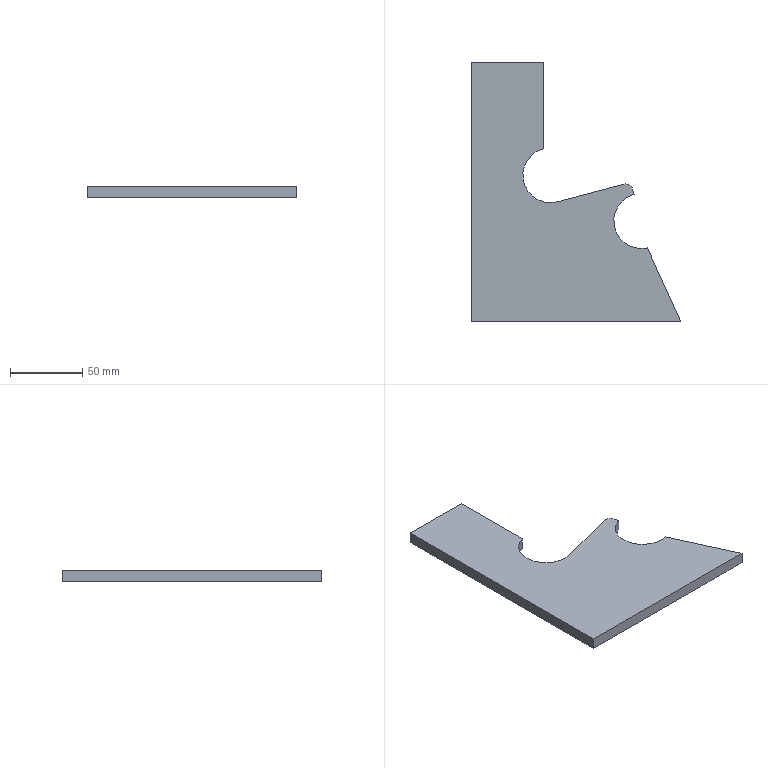Part | SolidWorks | features FlatPattern 1, SMBaseFlange 1, SheetMetal 1 | 1 solid | 12 faces | box 145.357 x 180 x 8 mm | volume 119080 mm3 | plane 9 | cylinder 3 | commonest cylinder face diameters 38.1 x2 10 x1
STEP:
#1=CARTESIAN_POINT('',(-250.138,75.285,0.));
#2=VERTEX_POINT('',#1);
#3=CARTESIAN_POINT('',(-250.138,-104.715,0.));
#4=VERTEX_POINT('',#3);
#5=CARTESIAN_POINT('',(-250.138,-104.715,0.));
#6=DIRECTION('',(0.,-1.,0.));
#7=VECTOR('',#6,1000.);
#8=LINE('',#5,#7);
#9=EDGE_CURVE('',#2,#4,#8,.T.);
#10=ORIENTED_EDGE('',*,*,#9,.F.);
#11=CARTESIAN_POINT('',(-250.138,75.285,-8.));
#12=VERTEX_POINT('',#11);
#13=CARTESIAN_POINT('',(-250.138,75.285,-8.));
#14=DIRECTION('',(0.,0.,1.));
#15=VECTOR('',#14,1000.);
#16=LINE('',#13,#15);
#17=EDGE_CURVE('',#12,#2,#16,.T.);
#18=ORIENTED_EDGE('',*,*,#17,.F.);
#19=CARTESIAN_POINT('',(-250.138,-104.715,-8.));
#20=VERTEX_POINT('',#19);
#21=CARTESIAN_POINT('',(-250.138,-104.715,-8.));
#22=DIRECTION('',(0.,-1.,0.));
#23=VECTOR('',#22,1000.);
#24=LINE('',#21,#23);
#25=EDGE_CURVE('',#12,#20,#24,.T.);
#26=ORIENTED_EDGE('',*,*,#25,.T.);
#27=CARTESIAN_POINT('',(-250.138,-104.715,-8.));
#28=DIRECTION('',(0.,0.,1.));
#29=VECTOR('',#28,1000.);
#30=LINE('',#27,#29);
#31=EDGE_CURVE('',#20,#4,#30,.T.);
#32=ORIENTED_EDGE('',*,*,#31,.T.);
#33=EDGE_LOOP('',(#10,#18,#26,#32));
#34=FACE_OUTER_BOUND('',#33,.T.);
#35=CARTESIAN_POINT('',(-250.138,-104.715,-8.));
#36=DIRECTION('',(-1.,0.,0.));
#37=DIRECTION('',(0.,0.,1.));
#38=AXIS2_PLACEMENT_3D('',#35,#36,#37);
#39=PLANE('',#38);
#40=ADVANCED_FACE('',(#34),#39,.T.);
#41=CARTESIAN_POINT('',(-200.138,75.285,0.));
#42=VERTEX_POINT('',#41);
#43=CARTESIAN_POINT('',(-250.138,75.285,0.));
#44=DIRECTION('',(-1.,0.,0.));
#45=VECTOR('',#44,1000.);
#46=LINE('',#43,#45);
#47=EDGE_CURVE('',#42,#2,#46,.T.);
#48=ORIENTED_EDGE('',*,*,#47,.F.);
#49=CARTESIAN_POINT('',(-200.138,75.285,-8.));
#50=VERTEX_POINT('',#49);
#51=CARTESIAN_POINT('',(-200.138,75.285,-8.));
#52=DIRECTION('',(0.,0.,1.));
#53=VECTOR('',#52,1000.);
#54=LINE('',#51,#53);
#55=EDGE_CURVE('',#50,#42,#54,.T.);
#56=ORIENTED_EDGE('',*,*,#55,.F.);
#57=CARTESIAN_POINT('',(-250.138,75.285,-8.));
#58=DIRECTION('',(-1.,0.,0.));
#59=VECTOR('',#58,1000.);
#60=LINE('',#57,#59);
#61=EDGE_CURVE('',#50,#12,#60,.T.);
#62=ORIENTED_EDGE('',*,*,#61,.T.);
#63=ORIENTED_EDGE('',*,*,#17,.T.);
#64=EDGE_LOOP('',(#48,#56,#62,#63));
#65=FACE_OUTER_BOUND('',#64,.T.);
#66=CARTESIAN_POINT('',(-250.138,75.285,-8.));
#67=DIRECTION('',(0.,1.,0.));
#68=DIRECTION('',(0.,0.,1.));
#69=AXIS2_PLACEMENT_3D('',#66,#67,#68);
#70=PLANE('',#69);
#71=ADVANCED_FACE('',(#65),#70,.T.);
#72=CARTESIAN_POINT('',(-200.138,15.285,0.));
#73=VERTEX_POINT('',#72);
#74=CARTESIAN_POINT('',(-200.138,75.285,0.));
#75=DIRECTION('',(0.,1.,0.));
#76=VECTOR('',#75,1000.);
#77=LINE('',#74,#76);
#78=EDGE_CURVE('',#73,#42,#77,.T.);
#79=ORIENTED_EDGE('',*,*,#78,.F.);
#80=CARTESIAN_POINT('',(-200.138,15.285,-8.));
#81=VERTEX_POINT('',#80);
#82=CARTESIAN_POINT('',(-200.138,15.285,-8.));
#83=DIRECTION('',(0.,0.,1.));
#84=VECTOR('',#83,1000.);
#85=LINE('',#82,#84);
#86=EDGE_CURVE('',#81,#73,#85,.T.);
#87=ORIENTED_EDGE('',*,*,#86,.F.);
#88=CARTESIAN_POINT('',(-200.138,75.285,-8.));
#89=DIRECTION('',(0.,1.,0.));
#90=VECTOR('',#89,1000.);
#91=LINE('',#88,#90);
#92=EDGE_CURVE('',#81,#50,#91,.T.);
#93=ORIENTED_EDGE('',*,*,#92,.T.);
#94=ORIENTED_EDGE('',*,*,#55,.T.);
#95=EDGE_LOOP('',(#79,#87,#93,#94));
#96=FACE_OUTER_BOUND('',#95,.T.);
#97=CARTESIAN_POINT('',(-200.138,75.285,-8.));
#98=DIRECTION('',(1.,0.,0.));
#99=DIRECTION('',(0.,0.,-1.));
#100=AXIS2_PLACEMENT_3D('',#97,#98,#99);
#101=PLANE('',#100);
#102=ADVANCED_FACE('',(#96),#101,.T.);
#103=CARTESIAN_POINT('',(-190.368,-21.541,0.));
#104=VERTEX_POINT('',#103);
#105=CARTESIAN_POINT('',(-195.253,-3.128,0.));
#106=DIRECTION('',(0.,0.,-1.));
#107=DIRECTION('',(1.,0.,0.));
#108=AXIS2_PLACEMENT_3D('',#105,#106,#107);
#109=CIRCLE('',#108,19.05);
#110=EDGE_CURVE('',#104,#73,#109,.T.);
#111=ORIENTED_EDGE('',*,*,#110,.F.);
#112=CARTESIAN_POINT('',(-190.368,-21.541,-8.));
#113=VERTEX_POINT('',#112);
#114=CARTESIAN_POINT('',(-190.368,-21.541,-8.));
#115=DIRECTION('',(0.,0.,1.));
#116=VECTOR('',#115,1000.);
#117=LINE('',#114,#116);
#118=EDGE_CURVE('',#113,#104,#117,.T.);
#119=ORIENTED_EDGE('',*,*,#118,.F.);
#120=CARTESIAN_POINT('',(-195.253,-3.128,-8.));
#121=DIRECTION('',(0.,0.,-1.));
#122=DIRECTION('',(1.,0.,0.));
#123=AXIS2_PLACEMENT_3D('',#120,#121,#122);
#124=CIRCLE('',#123,19.05);
#125=EDGE_CURVE('',#113,#81,#124,.T.);
#126=ORIENTED_EDGE('',*,*,#125,.T.);
#127=ORIENTED_EDGE('',*,*,#86,.T.);
#128=EDGE_LOOP('',(#111,#119,#126,#127));
#129=FACE_OUTER_BOUND('',#128,.T.);
#130=CARTESIAN_POINT('',(-195.253,-3.128,-8.));
#131=DIRECTION('',(0.,0.,1.));
#132=DIRECTION('',(1.,0.,0.));
#133=AXIS2_PLACEMENT_3D('',#130,#131,#132);
#134=CYLINDRICAL_SURFACE('',#133,19.05);
#135=ADVANCED_FACE('',(#129),#134,.F.);
#136=CARTESIAN_POINT('',(-144.339,-9.329,0.));
#137=VERTEX_POINT('',#136);
#138=CARTESIAN_POINT('',(-190.368,-21.541,0.));
#139=DIRECTION('',(-0.9666,-0.2564,0.));
#140=VECTOR('',#139,1000.);
#141=LINE('',#138,#140);
#142=EDGE_CURVE('',#137,#104,#141,.T.);
#143=ORIENTED_EDGE('',*,*,#142,.F.);
#144=CARTESIAN_POINT('',(-144.339,-9.329,-8.));
#145=VERTEX_POINT('',#144);
#146=CARTESIAN_POINT('',(-144.339,-9.329,-8.));
#147=DIRECTION('',(0.,0.,1.));
#148=VECTOR('',#147,1000.);
#149=LINE('',#146,#148);
#150=EDGE_CURVE('',#145,#137,#149,.T.);
#151=ORIENTED_EDGE('',*,*,#150,.F.);
#152=CARTESIAN_POINT('',(-190.368,-21.541,-8.));
#153=DIRECTION('',(-0.9666,-0.2564,0.));
#154=VECTOR('',#153,1000.);
#155=LINE('',#152,#154);
#156=EDGE_CURVE('',#145,#113,#155,.T.);
#157=ORIENTED_EDGE('',*,*,#156,.T.);
#158=ORIENTED_EDGE('',*,*,#118,.T.);
#159=EDGE_LOOP('',(#143,#151,#157,#158));
#160=FACE_OUTER_BOUND('',#159,.T.);
#161=CARTESIAN_POINT('',(-190.368,-21.541,-8.));
#162=DIRECTION('',(-0.2564,0.9666,0.));
#163=DIRECTION('',(-0.9666,-0.2564,0.));
#164=AXIS2_PLACEMENT_3D('',#161,#162,#163);
#165=PLANE('',#164);
#166=ADVANCED_FACE('',(#160),#165,.T.);
#167=CARTESIAN_POINT('',(-138.224,-12.88,0.));
#168=VERTEX_POINT('',#167);
#169=CARTESIAN_POINT('',(-143.057,-14.162,0.));
#170=DIRECTION('',(0.,0.,1.));
#171=DIRECTION('',(-1.,0.,0.));
#172=AXIS2_PLACEMENT_3D('',#169,#170,#171);
#173=CIRCLE('',#172,5.);
#174=EDGE_CURVE('',#168,#137,#173,.T.);
#175=ORIENTED_EDGE('',*,*,#174,.F.);
#176=CARTESIAN_POINT('',(-138.224,-12.88,-8.));
#177=VERTEX_POINT('',#176);
#178=CARTESIAN_POINT('',(-138.224,-12.88,-8.));
#179=DIRECTION('',(0.,0.,1.));
#180=VECTOR('',#179,1000.);
#181=LINE('',#178,#180);
#182=EDGE_CURVE('',#177,#168,#181,.T.);
#183=ORIENTED_EDGE('',*,*,#182,.F.);
#184=CARTESIAN_POINT('',(-143.057,-14.162,-8.));
#185=DIRECTION('',(0.,0.,1.));
#186=DIRECTION('',(-1.,0.,0.));
#187=AXIS2_PLACEMENT_3D('',#184,#185,#186);
#188=CIRCLE('',#187,5.);
#189=EDGE_CURVE('',#177,#145,#188,.T.);
#190=ORIENTED_EDGE('',*,*,#189,.T.);
#191=ORIENTED_EDGE('',*,*,#150,.T.);
#192=EDGE_LOOP('',(#175,#183,#190,#191));
#193=FACE_OUTER_BOUND('',#192,.T.);
#194=CARTESIAN_POINT('',(-143.057,-14.162,-8.));
#195=DIRECTION('',(0.,0.,1.));
#196=DIRECTION('',(1.,0.,0.));
#197=AXIS2_PLACEMENT_3D('',#194,#195,#196);
#198=CYLINDRICAL_SURFACE('',#197,5.);
#199=ADVANCED_FACE('',(#193),#198,.T.);
#200=CARTESIAN_POINT('',(-137.264,-16.5,0.));
#201=VERTEX_POINT('',#200);
#202=CARTESIAN_POINT('',(-137.264,-16.5,0.));
#203=DIRECTION('',(-0.2564,0.9666,0.));
#204=VECTOR('',#203,1000.);
#205=LINE('',#202,#204);
#206=EDGE_CURVE('',#201,#168,#205,.T.);
#207=ORIENTED_EDGE('',*,*,#206,.F.);
#208=CARTESIAN_POINT('',(-137.264,-16.5,-8.));
#209=VERTEX_POINT('',#208);
#210=CARTESIAN_POINT('',(-137.264,-16.5,-8.));
#211=DIRECTION('',(0.,0.,1.));
#212=VECTOR('',#211,1000.);
#213=LINE('',#210,#212);
#214=EDGE_CURVE('',#209,#201,#213,.T.);
#215=ORIENTED_EDGE('',*,*,#214,.F.);
#216=CARTESIAN_POINT('',(-137.264,-16.5,-8.));
#217=DIRECTION('',(-0.2564,0.9666,0.));
#218=VECTOR('',#217,1000.);
#219=LINE('',#216,#218);
#220=EDGE_CURVE('',#209,#177,#219,.T.);
#221=ORIENTED_EDGE('',*,*,#220,.T.);
#222=ORIENTED_EDGE('',*,*,#182,.T.);
#223=EDGE_LOOP('',(#207,#215,#221,#222));
#224=FACE_OUTER_BOUND('',#223,.T.);
#225=CARTESIAN_POINT('',(-137.264,-16.5,-8.));
#226=DIRECTION('',(0.9666,0.2564,0.));
#227=DIRECTION('',(-0.2564,0.9666,0.));
#228=AXIS2_PLACEMENT_3D('',#225,#226,#227);
#229=PLANE('',#228);
#230=ADVANCED_FACE('',(#224),#229,.T.);
#231=CARTESIAN_POINT('',(-128.031,-53.453,0.));
#232=VERTEX_POINT('',#231);
#233=CARTESIAN_POINT('',(-132.208,-34.866,0.));
#234=DIRECTION('',(0.,0.,-1.));
#235=DIRECTION('',(1.,0.,0.));
#236=AXIS2_PLACEMENT_3D('',#233,#234,#235);
#237=CIRCLE('',#236,19.05);
#238=EDGE_CURVE('',#232,#201,#237,.T.);
#239=ORIENTED_EDGE('',*,*,#238,.F.);
#240=CARTESIAN_POINT('',(-128.031,-53.453,-8.));
#241=VERTEX_POINT('',#240);
#242=CARTESIAN_POINT('',(-128.031,-53.453,-8.));
#243=DIRECTION('',(0.,0.,1.));
#244=VECTOR('',#243,1000.);
#245=LINE('',#242,#244);
#246=EDGE_CURVE('',#241,#232,#245,.T.);
#247=ORIENTED_EDGE('',*,*,#246,.F.);
#248=CARTESIAN_POINT('',(-132.208,-34.866,-8.));
#249=DIRECTION('',(0.,0.,-1.));
#250=DIRECTION('',(1.,0.,0.));
#251=AXIS2_PLACEMENT_3D('',#248,#249,#250);
#252=CIRCLE('',#251,19.05);
#253=EDGE_CURVE('',#241,#209,#252,.T.);
#254=ORIENTED_EDGE('',*,*,#253,.T.);
#255=ORIENTED_EDGE('',*,*,#214,.T.);
#256=EDGE_LOOP('',(#239,#247,#254,#255));
#257=FACE_OUTER_BOUND('',#256,.T.);
#258=CARTESIAN_POINT('',(-132.208,-34.866,-8.));
#259=DIRECTION('',(0.,0.,1.));
#260=DIRECTION('',(1.,0.,0.));
#261=AXIS2_PLACEMENT_3D('',#258,#259,#260);
#262=CYLINDRICAL_SURFACE('',#261,19.05);
#263=ADVANCED_FACE('',(#257),#262,.F.);
#264=CARTESIAN_POINT('',(-104.781,-104.715,0.));
#265=VERTEX_POINT('',#264);
#266=CARTESIAN_POINT('',(-128.031,-53.453,0.));
#267=DIRECTION('',(-0.413,0.9107,0.));
#268=VECTOR('',#267,1000.);
#269=LINE('',#266,#268);
#270=EDGE_CURVE('',#265,#232,#269,.T.);
#271=ORIENTED_EDGE('',*,*,#270,.F.);
#272=CARTESIAN_POINT('',(-104.781,-104.715,-8.));
#273=VERTEX_POINT('',#272);
#274=CARTESIAN_POINT('',(-104.781,-104.715,-8.));
#275=DIRECTION('',(0.,0.,1.));
#276=VECTOR('',#275,1000.);
#277=LINE('',#274,#276);
#278=EDGE_CURVE('',#273,#265,#277,.T.);
#279=ORIENTED_EDGE('',*,*,#278,.F.);
#280=CARTESIAN_POINT('',(-128.031,-53.453,-8.));
#281=DIRECTION('',(-0.413,0.9107,0.));
#282=VECTOR('',#281,1000.);
#283=LINE('',#280,#282);
#284=EDGE_CURVE('',#273,#241,#283,.T.);
#285=ORIENTED_EDGE('',*,*,#284,.T.);
#286=ORIENTED_EDGE('',*,*,#246,.T.);
#287=EDGE_LOOP('',(#271,#279,#285,#286));
#288=FACE_OUTER_BOUND('',#287,.T.);
#289=CARTESIAN_POINT('',(-128.031,-53.453,-8.));
#290=DIRECTION('',(0.9107,0.413,0.));
#291=DIRECTION('',(-0.413,0.9107,0.));
#292=AXIS2_PLACEMENT_3D('',#289,#290,#291);
#293=PLANE('',#292);
#294=ADVANCED_FACE('',(#288),#293,.T.);
#295=CARTESIAN_POINT('',(-104.781,-104.715,0.));
#296=DIRECTION('',(1.,0.,0.));
#297=VECTOR('',#296,1000.);
#298=LINE('',#295,#297);
#299=EDGE_CURVE('',#4,#265,#298,.T.);
#300=ORIENTED_EDGE('',*,*,#299,.F.);
#301=ORIENTED_EDGE('',*,*,#31,.F.);
#302=CARTESIAN_POINT('',(-125.138,-104.715,-8.));
#303=DIRECTION('',(1.,0.,0.));
#304=VECTOR('',#303,1000.);
#305=LINE('',#302,#304);
#306=EDGE_CURVE('',#20,#273,#305,.T.);
#307=ORIENTED_EDGE('',*,*,#306,.T.);
#308=ORIENTED_EDGE('',*,*,#278,.T.);
#309=EDGE_LOOP('',(#300,#301,#307,#308));
#310=FACE_OUTER_BOUND('',#309,.T.);
#311=CARTESIAN_POINT('',(-104.781,-104.715,-8.));
#312=DIRECTION('',(0.,-1.,0.));
#313=DIRECTION('',(1.,0.,0.));
#314=AXIS2_PLACEMENT_3D('',#311,#312,#313);
#315=PLANE('',#314);
#316=ADVANCED_FACE('',(#310),#315,.T.);
#317=ORIENTED_EDGE('',*,*,#25,.F.);
#318=ORIENTED_EDGE('',*,*,#61,.F.);
#319=ORIENTED_EDGE('',*,*,#92,.F.);
#320=ORIENTED_EDGE('',*,*,#125,.F.);
#321=ORIENTED_EDGE('',*,*,#156,.F.);
#322=ORIENTED_EDGE('',*,*,#189,.F.);
#323=ORIENTED_EDGE('',*,*,#220,.F.);
#324=ORIENTED_EDGE('',*,*,#253,.F.);
#325=ORIENTED_EDGE('',*,*,#284,.F.);
#326=ORIENTED_EDGE('',*,*,#306,.F.);
#327=EDGE_LOOP('',(#317,#318,#319,#320,#321,#322,#323,#324,#325,#326));
#328=FACE_OUTER_BOUND('',#327,.T.);
#329=CARTESIAN_POINT('',(-195.253,-3.128,-8.));
#330=DIRECTION('',(0.,0.,1.));
#331=DIRECTION('',(1.,0.,0.));
#332=AXIS2_PLACEMENT_3D('',#329,#330,#331);
#333=PLANE('',#332);
#334=ADVANCED_FACE('',(#328),#333,.F.);
#335=ORIENTED_EDGE('',*,*,#9,.T.);
#336=ORIENTED_EDGE('',*,*,#299,.T.);
#337=ORIENTED_EDGE('',*,*,#270,.T.);
#338=ORIENTED_EDGE('',*,*,#238,.T.);
#339=ORIENTED_EDGE('',*,*,#206,.T.);
#340=ORIENTED_EDGE('',*,*,#174,.T.);
#341=ORIENTED_EDGE('',*,*,#142,.T.);
#342=ORIENTED_EDGE('',*,*,#110,.T.);
#343=ORIENTED_EDGE('',*,*,#78,.T.);
#344=ORIENTED_EDGE('',*,*,#47,.T.);
#345=EDGE_LOOP('',(#335,#336,#337,#338,#339,#340,#341,#342,#343,#344));
#346=FACE_OUTER_BOUND('',#345,.T.);
#347=CARTESIAN_POINT('',(-195.253,-3.128,0.));
#348=DIRECTION('',(0.,0.,1.));
#349=DIRECTION('',(1.,0.,0.));
#350=AXIS2_PLACEMENT_3D('',#347,#348,#349);
#351=PLANE('',#350);
#352=ADVANCED_FACE('',(#346),#351,.T.);
#353=CLOSED_SHELL('',(#40,#71,#102,#135,#166,#199,#230,#263,#294,#316,#334,#352));
#354=MANIFOLD_SOLID_BREP('',#353);
#355=CARTESIAN_POINT('',(0.,0.,0.));
#356=DIRECTION('',(0.,0.,1.));
#357=DIRECTION('',(1.,0.,0.));
#358=AXIS2_PLACEMENT_3D('',#355,#356,#357);
#359=(LENGTH_UNIT()NAMED_UNIT(*)SI_UNIT(.MILLI.,.METRE.));
#360=UNCERTAINTY_MEASURE_WITH_UNIT(LENGTH_MEASURE(0.00001),#359,'','');
#361=(NAMED_UNIT(*)PLANE_ANGLE_UNIT()SI_UNIT($,.RADIAN.));
#362=(NAMED_UNIT(*)SI_UNIT($,.STERADIAN.)SOLID_ANGLE_UNIT());
#363=(GEOMETRIC_REPRESENTATION_CONTEXT(3)GLOBAL_UNCERTAINTY_ASSIGNED_CONTEXT((#360))GLOBAL_UNIT_ASSIGNED_CONTEXT((#359,#361,#362))REPRESENTATION_CONTEXT('',''));
#364=ADVANCED_BREP_SHAPE_REPRESENTATION('',(#354,#358),#363);